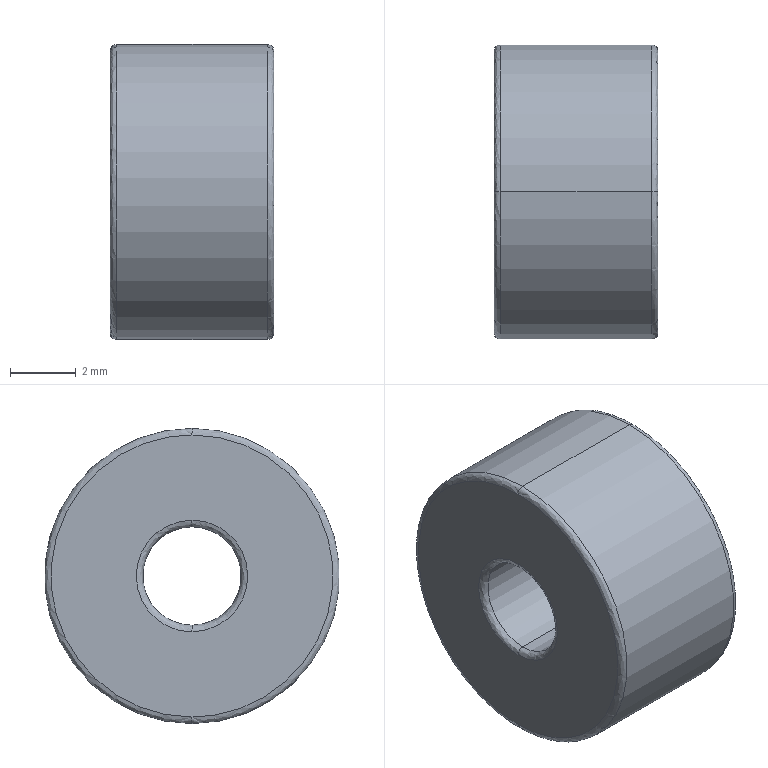Part | STEP file | Bearing B603ZZ | 1 solid | 14 faces | box 5 x 9 x 9 mm | volume 282.092 mm3 | spline 8 | cylinder 4 | plane 2 | commonest cylinder face diameters 3 x2 9 x2